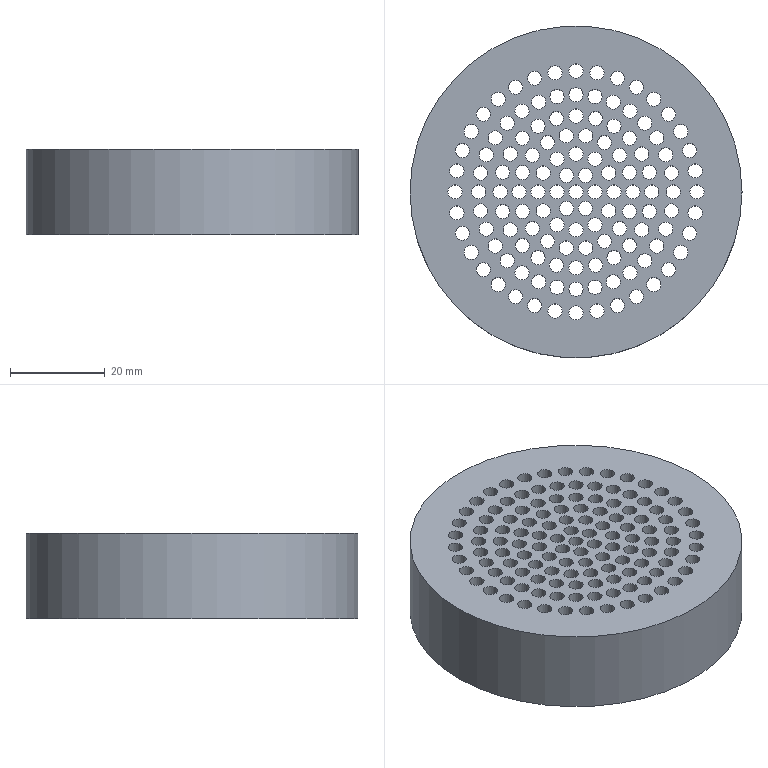CAM job | NX | drilling | part box 70 x 70 x 18 mm | stock box 33260 x 24047 x 18 mm
Tools:
number,name,description,diameter,corner_radius,flute_length,length,flutes
1,ZXZ,Milling Tool-5 Parameters,6.0,0.0,50.0,75.0,2
7,D6A45,Milling Tool-5 Parameters,6.0,0.0,50.0,75.0,2
13,3.0ZT,Drilling Tool,3.0,0.0,35.0,50.0,2
12,2.5ZT,Drilling Tool,2.5,0.0,35.0,50.0,2
Operations:
program,operation,operation_type,tool,method,geometry_group,spindle_rpm,surface_speed,feed_per_tooth,feed_cut,feed_plunge,cut_length_mm,path_length_mm,cut_time_min,machine_time_min
1,DRILLING,Operation,ZXZ,METHOD,A,3000.0,56.0,0.0417,250.0,0.0,516.0,2138.942,2.064,2.226
1,DRILLING_COPY,Operation,3.0ZT,METHOD,A,2971.0,28.0,0.0202,120.0,0.0,2954.267,7015.475,24.619,25.025
1,DRILLING_COPY_1,Operation,D6A45,METHOD,A,3000.0,56.0,0.0417,250.0,0.0,593.4,2293.742,2.374,2.544
D60,DRILLING_COPY_2,Operation,ZXZ,METHOD,A,3000.0,56.0,0.0417,250.0,0.0,372.0,1548.054,1.488,1.606
D60,DRILLING_COPY_COPY,Operation,2.5ZT,METHOD,A,2971.0,28.0,0.0202,120.0,0.0,2115.85,5035.755,17.632,17.924
D60,DRILLING_COPY_1_COPY,Operation,D6A45,METHOD,A,3000.0,56.0,0.0417,250.0,0.0,404.55,1613.155,1.618,1.739